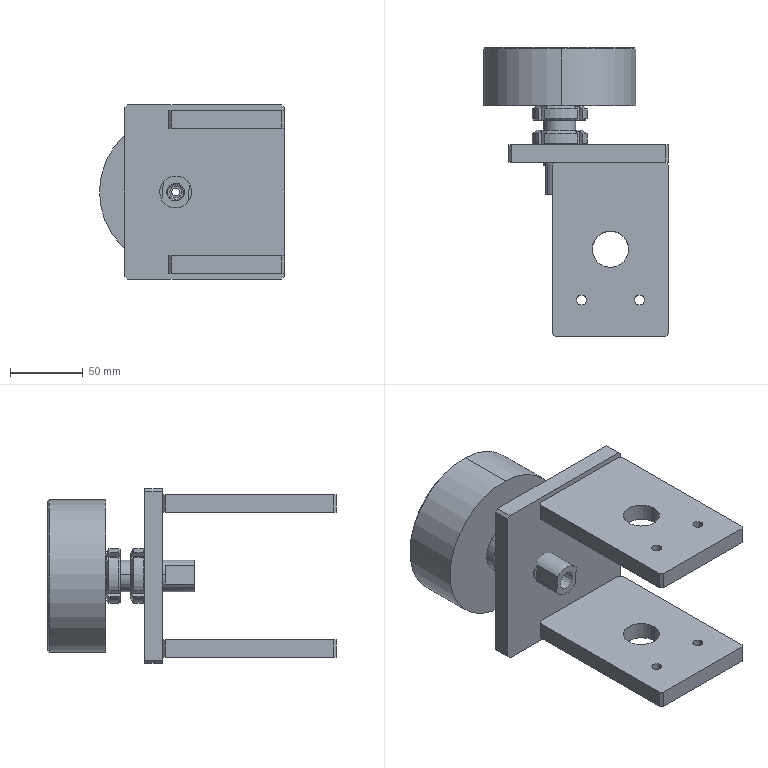Part | SolidWorks | 7 solids | 247 faces | box 127.5 x 199 x 120 mm | volume 502841 mm3 | plane 83 | cylinder 82 | cone 55 | spline 25 | torus 2 | commonest cylinder face diameters 6.8 x16 5.2 x8 9 x8 15 x8 38 x8 22 x6